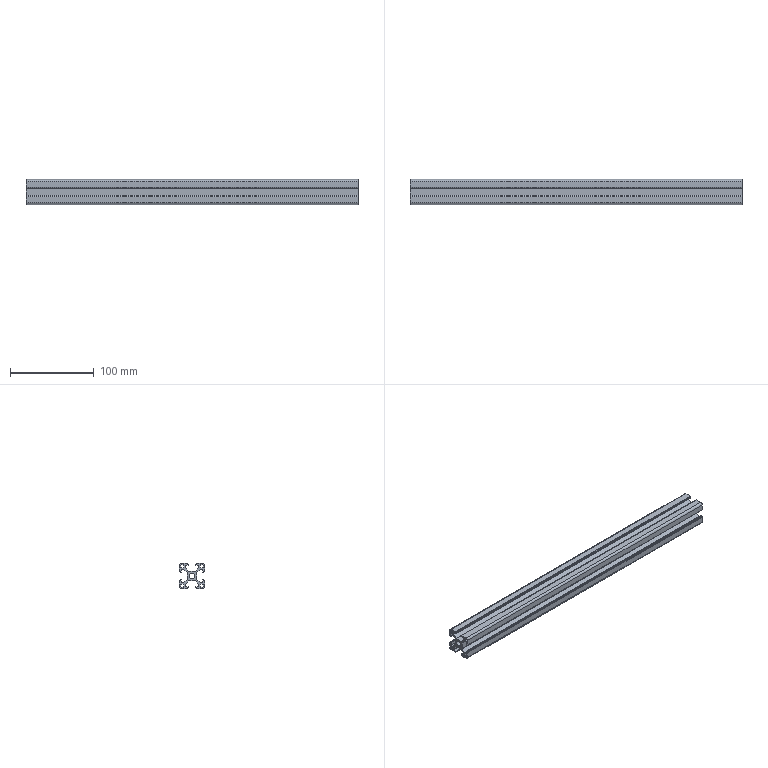Part | STEP file | 1 solid | 163 faces | box 397 x 30 x 30 mm | volume 129616 mm3 | cylinder 81 | plane 78 | cone 4 | commonest cylinder face diameters 0.6 x55 2 x16 5 x4 6.9 x4 6.8 x2